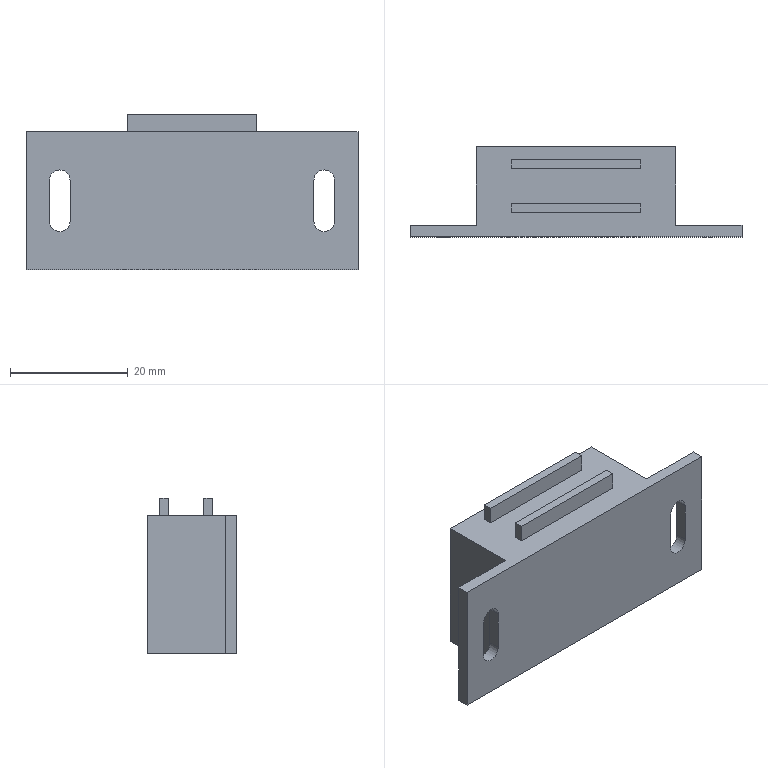Part | SolidWorks | features BaseBody 1 | 1 solid | 30 faces | box 56.5 x 15.3 x 26.5 mm | volume 13344 mm3 | plane 24 | cylinder 6 | commonest cylinder face diameters 3.5 x6
STEP:
#1=CARTESIAN_POINT('',(-20.75,0.,3.5));
#2=VERTEX_POINT('',#1);
#3=CARTESIAN_POINT('',(-22.5,0.,5.25));
#4=VERTEX_POINT('',#3);
#5=CARTESIAN_POINT('',(-22.5,0.,3.5));
#6=DIRECTION('',(0.,-1.,0.));
#7=DIRECTION('',(0.,0.,1.));
#8=AXIS2_PLACEMENT_3D('',#5,#6,#7);
#9=CIRCLE('',#8,1.75);
#10=EDGE_CURVE('',#2,#4,#9,.T.);
#11=ORIENTED_EDGE('',*,*,#10,.T.);
#12=CARTESIAN_POINT('',(-22.5,2.,5.25));
#13=VERTEX_POINT('',#12);
#14=CARTESIAN_POINT('',(-22.5,0.,5.25));
#15=DIRECTION('',(0.,1.,0.));
#16=VECTOR('',#15,1000.);
#17=LINE('',#14,#16);
#18=EDGE_CURVE('',#4,#13,#17,.T.);
#19=ORIENTED_EDGE('',*,*,#18,.T.);
#20=CARTESIAN_POINT('',(-20.75,2.,3.5));
#21=VERTEX_POINT('',#20);
#22=CARTESIAN_POINT('',(-22.5,2.,3.5));
#23=DIRECTION('',(0.,-1.,0.));
#24=DIRECTION('',(0.,0.,1.));
#25=AXIS2_PLACEMENT_3D('',#22,#23,#24);
#26=CIRCLE('',#25,1.75);
#27=EDGE_CURVE('',#21,#13,#26,.T.);
#28=ORIENTED_EDGE('',*,*,#27,.F.);
#29=CARTESIAN_POINT('',(-20.75,0.,3.5));
#30=DIRECTION('',(0.,-1.,0.));
#31=VECTOR('',#30,1000.);
#32=LINE('',#29,#31);
#33=EDGE_CURVE('',#21,#2,#32,.T.);
#34=ORIENTED_EDGE('',*,*,#33,.T.);
#35=EDGE_LOOP('',(#11,#19,#28,#34));
#36=FACE_OUTER_BOUND('',#35,.T.);
#37=CARTESIAN_POINT('',(-22.5,0.,3.5));
#38=DIRECTION('',(0.,1.,0.));
#39=DIRECTION('',(0.,0.,1.));
#40=AXIS2_PLACEMENT_3D('',#37,#38,#39);
#41=CYLINDRICAL_SURFACE('',#40,1.75);
#42=ADVANCED_FACE('',(#36),#41,.F.);
#43=CARTESIAN_POINT('',(24.25,0.,3.5));
#44=VERTEX_POINT('',#43);
#45=CARTESIAN_POINT('',(22.5,0.,5.25));
#46=VERTEX_POINT('',#45);
#47=CARTESIAN_POINT('',(22.5,0.,3.5));
#48=DIRECTION('',(0.,-1.,0.));
#49=DIRECTION('',(0.,0.,1.));
#50=AXIS2_PLACEMENT_3D('',#47,#48,#49);
#51=CIRCLE('',#50,1.75);
#52=EDGE_CURVE('',#44,#46,#51,.T.);
#53=ORIENTED_EDGE('',*,*,#52,.T.);
#54=CARTESIAN_POINT('',(22.5,2.,5.25));
#55=VERTEX_POINT('',#54);
#56=CARTESIAN_POINT('',(22.5,0.,5.25));
#57=DIRECTION('',(0.,1.,0.));
#58=VECTOR('',#57,1000.);
#59=LINE('',#56,#58);
#60=EDGE_CURVE('',#46,#55,#59,.T.);
#61=ORIENTED_EDGE('',*,*,#60,.T.);
#62=CARTESIAN_POINT('',(24.25,2.,3.5));
#63=VERTEX_POINT('',#62);
#64=CARTESIAN_POINT('',(22.5,2.,3.5));
#65=DIRECTION('',(0.,-1.,0.));
#66=DIRECTION('',(0.,0.,1.));
#67=AXIS2_PLACEMENT_3D('',#64,#65,#66);
#68=CIRCLE('',#67,1.75);
#69=EDGE_CURVE('',#63,#55,#68,.T.);
#70=ORIENTED_EDGE('',*,*,#69,.F.);
#71=CARTESIAN_POINT('',(24.25,0.,3.5));
#72=DIRECTION('',(0.,-1.,0.));
#73=VECTOR('',#72,1000.);
#74=LINE('',#71,#73);
#75=EDGE_CURVE('',#63,#44,#74,.T.);
#76=ORIENTED_EDGE('',*,*,#75,.T.);
#77=EDGE_LOOP('',(#53,#61,#70,#76));
#78=FACE_OUTER_BOUND('',#77,.T.);
#79=CARTESIAN_POINT('',(22.5,0.,3.5));
#80=DIRECTION('',(0.,1.,0.));
#81=DIRECTION('',(0.,0.,1.));
#82=AXIS2_PLACEMENT_3D('',#79,#80,#81);
#83=CYLINDRICAL_SURFACE('',#82,1.75);
#84=ADVANCED_FACE('',(#78),#83,.F.);
#85=CARTESIAN_POINT('',(-28.25,0.,11.75));
#86=VERTEX_POINT('',#85);
#87=CARTESIAN_POINT('',(28.25,0.,11.75));
#88=VERTEX_POINT('',#87);
#89=CARTESIAN_POINT('',(0.,0.,11.75));
#90=DIRECTION('',(1.,0.,0.));
#91=VECTOR('',#90,1000.);
#92=LINE('',#89,#91);
#93=EDGE_CURVE('',#86,#88,#92,.T.);
#94=ORIENTED_EDGE('',*,*,#93,.F.);
#95=CARTESIAN_POINT('',(-28.25,0.,-11.75));
#96=VERTEX_POINT('',#95);
#97=CARTESIAN_POINT('',(-28.25,0.,0.));
#98=DIRECTION('',(0.,0.,1.));
#99=VECTOR('',#98,1000.);
#100=LINE('',#97,#99);
#101=EDGE_CURVE('',#96,#86,#100,.T.);
#102=ORIENTED_EDGE('',*,*,#101,.F.);
#103=CARTESIAN_POINT('',(28.25,0.,-11.75));
#104=VERTEX_POINT('',#103);
#105=CARTESIAN_POINT('',(0.,0.,-11.75));
#106=DIRECTION('',(-1.,0.,0.));
#107=VECTOR('',#106,1000.);
#108=LINE('',#105,#107);
#109=EDGE_CURVE('',#104,#96,#108,.T.);
#110=ORIENTED_EDGE('',*,*,#109,.F.);
#111=CARTESIAN_POINT('',(28.25,0.,0.));
#112=DIRECTION('',(0.,0.,-1.));
#113=VECTOR('',#112,1000.);
#114=LINE('',#111,#113);
#115=EDGE_CURVE('',#88,#104,#114,.T.);
#116=ORIENTED_EDGE('',*,*,#115,.F.);
#117=EDGE_LOOP('',(#94,#102,#110,#116));
#118=FACE_OUTER_BOUND('',#117,.T.);
#119=CARTESIAN_POINT('',(-24.25,0.,-3.5));
#120=VERTEX_POINT('',#119);
#121=CARTESIAN_POINT('',(-20.75,0.,-3.5));
#122=VERTEX_POINT('',#121);
#123=CARTESIAN_POINT('',(-22.5,0.,-3.5));
#124=DIRECTION('',(0.,-1.,0.));
#125=DIRECTION('',(0.,0.,1.));
#126=AXIS2_PLACEMENT_3D('',#123,#124,#125);
#127=CIRCLE('',#126,1.75);
#128=EDGE_CURVE('',#120,#122,#127,.T.);
#129=ORIENTED_EDGE('',*,*,#128,.F.);
#130=CARTESIAN_POINT('',(-24.25,0.,3.5));
#131=VERTEX_POINT('',#130);
#132=CARTESIAN_POINT('',(-24.25,0.,0.));
#133=DIRECTION('',(0.,0.,-1.));
#134=VECTOR('',#133,1000.);
#135=LINE('',#132,#134);
#136=EDGE_CURVE('',#131,#120,#135,.T.);
#137=ORIENTED_EDGE('',*,*,#136,.F.);
#138=CARTESIAN_POINT('',(-22.5,0.,3.5));
#139=DIRECTION('',(0.,-1.,0.));
#140=DIRECTION('',(0.,0.,1.));
#141=AXIS2_PLACEMENT_3D('',#138,#139,#140);
#142=CIRCLE('',#141,1.75);
#143=EDGE_CURVE('',#4,#131,#142,.T.);
#144=ORIENTED_EDGE('',*,*,#143,.F.);
#145=ORIENTED_EDGE('',*,*,#10,.F.);
#146=CARTESIAN_POINT('',(-20.75,0.,0.));
#147=DIRECTION('',(0.,0.,1.));
#148=VECTOR('',#147,1000.);
#149=LINE('',#146,#148);
#150=EDGE_CURVE('',#122,#2,#149,.T.);
#151=ORIENTED_EDGE('',*,*,#150,.F.);
#152=EDGE_LOOP('',(#129,#137,#144,#145,#151));
#153=FACE_BOUND('',#152,.T.);
#154=CARTESIAN_POINT('',(20.75,0.,-3.5));
#155=VERTEX_POINT('',#154);
#156=CARTESIAN_POINT('',(24.25,0.,-3.5));
#157=VERTEX_POINT('',#156);
#158=CARTESIAN_POINT('',(22.5,0.,-3.5));
#159=DIRECTION('',(0.,-1.,0.));
#160=DIRECTION('',(0.,0.,1.));
#161=AXIS2_PLACEMENT_3D('',#158,#159,#160);
#162=CIRCLE('',#161,1.75);
#163=EDGE_CURVE('',#155,#157,#162,.T.);
#164=ORIENTED_EDGE('',*,*,#163,.F.);
#165=CARTESIAN_POINT('',(20.75,0.,3.5));
#166=VERTEX_POINT('',#165);
#167=CARTESIAN_POINT('',(20.75,0.,0.));
#168=DIRECTION('',(0.,0.,-1.));
#169=VECTOR('',#168,1000.);
#170=LINE('',#167,#169);
#171=EDGE_CURVE('',#166,#155,#170,.T.);
#172=ORIENTED_EDGE('',*,*,#171,.F.);
#173=CARTESIAN_POINT('',(22.5,0.,3.5));
#174=DIRECTION('',(0.,-1.,0.));
#175=DIRECTION('',(0.,0.,1.));
#176=AXIS2_PLACEMENT_3D('',#173,#174,#175);
#177=CIRCLE('',#176,1.75);
#178=EDGE_CURVE('',#46,#166,#177,.T.);
#179=ORIENTED_EDGE('',*,*,#178,.F.);
#180=ORIENTED_EDGE('',*,*,#52,.F.);
#181=CARTESIAN_POINT('',(24.25,0.,0.));
#182=DIRECTION('',(0.,0.,1.));
#183=VECTOR('',#182,1000.);
#184=LINE('',#181,#183);
#185=EDGE_CURVE('',#157,#44,#184,.T.);
#186=ORIENTED_EDGE('',*,*,#185,.F.);
#187=EDGE_LOOP('',(#164,#172,#179,#180,#186));
#188=FACE_BOUND('',#187,.T.);
#189=CARTESIAN_POINT('',(0.,0.,0.));
#190=DIRECTION('',(0.,1.,0.));
#191=DIRECTION('',(0.,0.,1.));
#192=AXIS2_PLACEMENT_3D('',#189,#190,#191);
#193=PLANE('',#192);
#194=ADVANCED_FACE('',(#118,#153,#188),#193,.F.);
#195=CARTESIAN_POINT('',(28.25,2.,-11.75));
#196=VERTEX_POINT('',#195);
#197=CARTESIAN_POINT('',(28.25,2.,-11.75));
#198=DIRECTION('',(0.,-1.,0.));
#199=VECTOR('',#198,1000.);
#200=LINE('',#197,#199);
#201=EDGE_CURVE('',#196,#104,#200,.T.);
#202=ORIENTED_EDGE('',*,*,#201,.F.);
#203=CARTESIAN_POINT('',(28.25,2.,11.75));
#204=VERTEX_POINT('',#203);
#205=CARTESIAN_POINT('',(28.25,2.,-11.75));
#206=DIRECTION('',(0.,0.,-1.));
#207=VECTOR('',#206,1000.);
#208=LINE('',#205,#207);
#209=EDGE_CURVE('',#204,#196,#208,.T.);
#210=ORIENTED_EDGE('',*,*,#209,.F.);
#211=CARTESIAN_POINT('',(28.25,2.,11.75));
#212=DIRECTION('',(0.,1.,0.));
#213=VECTOR('',#212,1000.);
#214=LINE('',#211,#213);
#215=EDGE_CURVE('',#88,#204,#214,.T.);
#216=ORIENTED_EDGE('',*,*,#215,.F.);
#217=ORIENTED_EDGE('',*,*,#115,.T.);
#218=EDGE_LOOP('',(#202,#210,#216,#217));
#219=FACE_OUTER_BOUND('',#218,.T.);
#220=CARTESIAN_POINT('',(28.25,2.,-11.75));
#221=DIRECTION('',(-1.,0.,0.));
#222=DIRECTION('',(0.,0.,1.));
#223=AXIS2_PLACEMENT_3D('',#220,#221,#222);
#224=PLANE('',#223);
#225=ADVANCED_FACE('',(#219),#224,.F.);
#226=CARTESIAN_POINT('',(11.,5.65,11.75));
#227=VERTEX_POINT('',#226);
#228=CARTESIAN_POINT('',(-11.,5.65,11.75));
#229=VERTEX_POINT('',#228);
#230=CARTESIAN_POINT('',(-28.25,5.65,11.75));
#231=DIRECTION('',(-1.,0.,0.));
#232=VECTOR('',#231,1000.);
#233=LINE('',#230,#232);
#234=EDGE_CURVE('',#227,#229,#233,.T.);
#235=ORIENTED_EDGE('',*,*,#234,.F.);
#236=CARTESIAN_POINT('',(11.,4.15,11.75));
#237=VERTEX_POINT('',#236);
#238=CARTESIAN_POINT('',(11.,4.15,11.75));
#239=DIRECTION('',(0.,-1.,0.));
#240=VECTOR('',#239,1000.);
#241=LINE('',#238,#240);
#242=EDGE_CURVE('',#227,#237,#241,.T.);
#243=ORIENTED_EDGE('',*,*,#242,.T.);
#244=CARTESIAN_POINT('',(-11.,4.15,11.75));
#245=VERTEX_POINT('',#244);
#246=CARTESIAN_POINT('',(-28.25,4.15,11.75));
#247=DIRECTION('',(1.,0.,0.));
#248=VECTOR('',#247,1000.);
#249=LINE('',#246,#248);
#250=EDGE_CURVE('',#245,#237,#249,.T.);
#251=ORIENTED_EDGE('',*,*,#250,.F.);
#252=CARTESIAN_POINT('',(-11.,4.15,11.75));
#253=DIRECTION('',(0.,1.,0.));
#254=VECTOR('',#253,1000.);
#255=LINE('',#252,#254);
#256=EDGE_CURVE('',#245,#229,#255,.T.);
#257=ORIENTED_EDGE('',*,*,#256,.T.);
#258=EDGE_LOOP('',(#235,#243,#251,#257));
#259=FACE_BOUND('',#258,.T.);
#260=ORIENTED_EDGE('',*,*,#215,.T.);
#261=CARTESIAN_POINT('',(17.,2.,11.75));
#262=VERTEX_POINT('',#261);
#263=CARTESIAN_POINT('',(-28.25,2.,11.75));
#264=DIRECTION('',(1.,0.,0.));
#265=VECTOR('',#264,1000.);
#266=LINE('',#263,#265);
#267=EDGE_CURVE('',#262,#204,#266,.T.);
#268=ORIENTED_EDGE('',*,*,#267,.F.);
#269=CARTESIAN_POINT('',(17.,15.3,11.75));
#270=VERTEX_POINT('',#269);
#271=CARTESIAN_POINT('',(17.,2.,11.75));
#272=DIRECTION('',(0.,-1.,0.));
#273=VECTOR('',#272,1000.);
#274=LINE('',#271,#273);
#275=EDGE_CURVE('',#270,#262,#274,.T.);
#276=ORIENTED_EDGE('',*,*,#275,.F.);
#277=CARTESIAN_POINT('',(-17.,15.3,11.75));
#278=VERTEX_POINT('',#277);
#279=CARTESIAN_POINT('',(-28.25,15.3,11.75));
#280=DIRECTION('',(1.,0.,0.));
#281=VECTOR('',#280,1000.);
#282=LINE('',#279,#281);
#283=EDGE_CURVE('',#278,#270,#282,.T.);
#284=ORIENTED_EDGE('',*,*,#283,.F.);
#285=CARTESIAN_POINT('',(-17.,2.,11.75));
#286=VERTEX_POINT('',#285);
#287=CARTESIAN_POINT('',(-17.,2.,11.75));
#288=DIRECTION('',(0.,1.,0.));
#289=VECTOR('',#288,1000.);
#290=LINE('',#287,#289);
#291=EDGE_CURVE('',#286,#278,#290,.T.);
#292=ORIENTED_EDGE('',*,*,#291,.F.);
#293=CARTESIAN_POINT('',(-28.25,2.,11.75));
#294=VERTEX_POINT('',#293);
#295=CARTESIAN_POINT('',(-28.25,2.,11.75));
#296=DIRECTION('',(1.,0.,0.));
#297=VECTOR('',#296,1000.);
#298=LINE('',#295,#297);
#299=EDGE_CURVE('',#294,#286,#298,.T.);
#300=ORIENTED_EDGE('',*,*,#299,.F.);
#301=CARTESIAN_POINT('',(-28.25,2.,11.75));
#302=DIRECTION('',(0.,1.,0.));
#303=VECTOR('',#302,1000.);
#304=LINE('',#301,#303);
#305=EDGE_CURVE('',#86,#294,#304,.T.);
#306=ORIENTED_EDGE('',*,*,#305,.F.);
#307=ORIENTED_EDGE('',*,*,#93,.T.);
#308=EDGE_LOOP('',(#260,#268,#276,#284,#292,#300,#306,#307));
#309=FACE_OUTER_BOUND('',#308,.T.);
#310=CARTESIAN_POINT('',(-11.,11.65,11.75));
#311=VERTEX_POINT('',#310);
#312=CARTESIAN_POINT('',(11.,11.65,11.75));
#313=VERTEX_POINT('',#312);
#314=CARTESIAN_POINT('',(-28.25,11.65,11.75));
#315=DIRECTION('',(1.,0.,0.));
#316=VECTOR('',#315,1000.);
#317=LINE('',#314,#316);
#318=EDGE_CURVE('',#311,#313,#317,.T.);
#319=ORIENTED_EDGE('',*,*,#318,.F.);
#320=CARTESIAN_POINT('',(-11.,13.15,11.75));
#321=VERTEX_POINT('',#320);
#322=CARTESIAN_POINT('',(-11.,13.15,11.75));
#323=DIRECTION('',(0.,1.,0.));
#324=VECTOR('',#323,1000.);
#325=LINE('',#322,#324);
#326=EDGE_CURVE('',#311,#321,#325,.T.);
#327=ORIENTED_EDGE('',*,*,#326,.T.);
#328=CARTESIAN_POINT('',(11.,13.15,11.75));
#329=VERTEX_POINT('',#328);
#330=CARTESIAN_POINT('',(-28.25,13.15,11.75));
#331=DIRECTION('',(-1.,0.,0.));
#332=VECTOR('',#331,1000.);
#333=LINE('',#330,#332);
#334=EDGE_CURVE('',#329,#321,#333,.T.);
#335=ORIENTED_EDGE('',*,*,#334,.F.);
#336=CARTESIAN_POINT('',(11.,13.15,11.75));
#337=DIRECTION('',(0.,-1.,0.));
#338=VECTOR('',#337,1000.);
#339=LINE('',#336,#338);
#340=EDGE_CURVE('',#329,#313,#339,.T.);
#341=ORIENTED_EDGE('',*,*,#340,.T.);
#342=EDGE_LOOP('',(#319,#327,#335,#341));
#343=FACE_BOUND('',#342,.T.);
#344=CARTESIAN_POINT('',(-28.25,2.,11.75));
#345=DIRECTION('',(0.,0.,-1.));
#346=DIRECTION('',(-1.,0.,0.));
#347=AXIS2_PLACEMENT_3D('',#344,#345,#346);
#348=PLANE('',#347);
#349=ADVANCED_FACE('',(#259,#309,#343),#348,.F.);
#350=ORIENTED_EDGE('',*,*,#305,.T.);
#351=CARTESIAN_POINT('',(-28.25,2.,-11.75));
#352=VERTEX_POINT('',#351);
#353=CARTESIAN_POINT('',(-28.25,2.,-11.75));
#354=DIRECTION('',(0.,0.,1.));
#355=VECTOR('',#354,1000.);
#356=LINE('',#353,#355);
#357=EDGE_CURVE('',#352,#294,#356,.T.);
#358=ORIENTED_EDGE('',*,*,#357,.F.);
#359=CARTESIAN_POINT('',(-28.25,2.,-11.75));
#360=DIRECTION('',(0.,1.,0.));
#361=VECTOR('',#360,1000.);
#362=LINE('',#359,#361);
#363=EDGE_CURVE('',#96,#352,#362,.T.);
#364=ORIENTED_EDGE('',*,*,#363,.F.);
#365=ORIENTED_EDGE('',*,*,#101,.T.);
#366=EDGE_LOOP('',(#350,#358,#364,#365));
#367=FACE_OUTER_BOUND('',#366,.T.);
#368=CARTESIAN_POINT('',(-28.25,2.,-11.75));
#369=DIRECTION('',(1.,0.,0.));
#370=DIRECTION('',(0.,0.,-1.));
#371=AXIS2_PLACEMENT_3D('',#368,#369,#370);
#372=PLANE('',#371);
#373=ADVANCED_FACE('',(#367),#372,.F.);
#374=ORIENTED_EDGE('',*,*,#363,.T.);
#375=CARTESIAN_POINT('',(-17.,2.,-11.75));
#376=VERTEX_POINT('',#375);
#377=CARTESIAN_POINT('',(-28.25,2.,-11.75));
#378=DIRECTION('',(-1.,0.,0.));
#379=VECTOR('',#378,1000.);
#380=LINE('',#377,#379);
#381=EDGE_CURVE('',#376,#352,#380,.T.);
#382=ORIENTED_EDGE('',*,*,#381,.F.);
#383=CARTESIAN_POINT('',(-17.,15.3,-11.75));
#384=VERTEX_POINT('',#383);
#385=CARTESIAN_POINT('',(-17.,2.,-11.75));
#386=DIRECTION('',(0.,-1.,0.));
#387=VECTOR('',#386,1000.);
#388=LINE('',#385,#387);
#389=EDGE_CURVE('',#384,#376,#388,.T.);
#390=ORIENTED_EDGE('',*,*,#389,.F.);
#391=CARTESIAN_POINT('',(17.,15.3,-11.75));
#392=VERTEX_POINT('',#391);
#393=CARTESIAN_POINT('',(-28.25,15.3,-11.75));
#394=DIRECTION('',(-1.,0.,0.));
#395=VECTOR('',#394,1000.);
#396=LINE('',#393,#395);
#397=EDGE_CURVE('',#392,#384,#396,.T.);
#398=ORIENTED_EDGE('',*,*,#397,.F.);
#399=CARTESIAN_POINT('',(17.,2.,-11.75));
#400=VERTEX_POINT('',#399);
#401=CARTESIAN_POINT('',(17.,2.,-11.75));
#402=DIRECTION('',(0.,1.,0.));
#403=VECTOR('',#402,1000.);
#404=LINE('',#401,#403);
#405=EDGE_CURVE('',#400,#392,#404,.T.);
#406=ORIENTED_EDGE('',*,*,#405,.F.);
#407=CARTESIAN_POINT('',(-28.25,2.,-11.75));
#408=DIRECTION('',(-1.,0.,0.));
#409=VECTOR('',#408,1000.);
#410=LINE('',#407,#409);
#411=EDGE_CURVE('',#196,#400,#410,.T.);
#412=ORIENTED_EDGE('',*,*,#411,.F.);
#413=ORIENTED_EDGE('',*,*,#201,.T.);
#414=ORIENTED_EDGE('',*,*,#109,.T.);
#415=EDGE_LOOP('',(#374,#382,#390,#398,#406,#412,#413,#414));
#416=FACE_OUTER_BOUND('',#415,.T.);
#417=CARTESIAN_POINT('',(-28.25,2.,-11.75));
#418=DIRECTION('',(0.,0.,1.));
#419=DIRECTION('',(1.,0.,0.));
#420=AXIS2_PLACEMENT_3D('',#417,#418,#419);
#421=PLANE('',#420);
#422=ADVANCED_FACE('',(#416),#421,.F.);
#423=CARTESIAN_POINT('',(-20.75,2.,-3.5));
#424=VERTEX_POINT('',#423);
#425=CARTESIAN_POINT('',(-20.75,0.,-3.5));
#426=DIRECTION('',(0.,1.,0.));
#427=VECTOR('',#426,1000.);
#428=LINE('',#425,#427);
#429=EDGE_CURVE('',#122,#424,#428,.T.);
#430=ORIENTED_EDGE('',*,*,#429,.F.);
#431=ORIENTED_EDGE('',*,*,#150,.T.);
#432=ORIENTED_EDGE('',*,*,#33,.F.);
#433=CARTESIAN_POINT('',(-20.75,2.,-3.5));
#434=DIRECTION('',(0.,0.,1.));
#435=VECTOR('',#434,1000.);
#436=LINE('',#433,#435);
#437=EDGE_CURVE('',#424,#21,#436,.T.);
#438=ORIENTED_EDGE('',*,*,#437,.F.);
#439=EDGE_LOOP('',(#430,#431,#432,#438));
#440=FACE_OUTER_BOUND('',#439,.T.);
#441=CARTESIAN_POINT('',(-20.75,0.,-3.5));
#442=DIRECTION('',(1.,0.,0.));
#443=DIRECTION('',(0.,0.,-1.));
#444=AXIS2_PLACEMENT_3D('',#441,#442,#443);
#445=PLANE('',#444);
#446=ADVANCED_FACE('',(#440),#445,.F.);
#447=CARTESIAN_POINT('',(-24.25,2.,-3.5));
#448=VERTEX_POINT('',#447);
#449=CARTESIAN_POINT('',(-24.25,0.,-3.5));
#450=DIRECTION('',(0.,1.,0.));
#451=VECTOR('',#450,1000.);
#452=LINE('',#449,#451);
#453=EDGE_CURVE('',#120,#448,#452,.T.);
#454=ORIENTED_EDGE('',*,*,#453,.F.);
#455=ORIENTED_EDGE('',*,*,#128,.T.);
#456=ORIENTED_EDGE('',*,*,#429,.T.);
#457=CARTESIAN_POINT('',(-22.5,2.,-3.5));
#458=DIRECTION('',(0.,-1.,0.));
#459=DIRECTION('',(0.,0.,1.));
#460=AXIS2_PLACEMENT_3D('',#457,#458,#459);
#461=CIRCLE('',#460,1.75);
#462=EDGE_CURVE('',#448,#424,#461,.T.);
#463=ORIENTED_EDGE('',*,*,#462,.F.);
#464=EDGE_LOOP('',(#454,#455,#456,#463));
#465=FACE_OUTER_BOUND('',#464,.T.);
#466=CARTESIAN_POINT('',(-22.5,0.,-3.5));
#467=DIRECTION('',(0.,1.,0.));
#468=DIRECTION('',(0.,0.,1.));
#469=AXIS2_PLACEMENT_3D('',#466,#467,#468);
#470=CYLINDRICAL_SURFACE('',#469,1.75);
#471=ADVANCED_FACE('',(#465),#470,.F.);
#472=CARTESIAN_POINT('',(-24.25,2.,3.5));
#473=VERTEX_POINT('',#472);
#474=CARTESIAN_POINT('',(-24.25,0.,3.5));
#475=DIRECTION('',(0.,1.,0.));
#476=VECTOR('',#475,1000.);
#477=LINE('',#474,#476);
#478=EDGE_CURVE('',#131,#473,#477,.T.);
#479=ORIENTED_EDGE('',*,*,#478,.F.);
#480=ORIENTED_EDGE('',*,*,#136,.T.);
#481=ORIENTED_EDGE('',*,*,#453,.T.);
#482=CARTESIAN_POINT('',(-24.25,2.,-3.5));
#483=DIRECTION('',(0.,0.,-1.));
#484=VECTOR('',#483,1000.);
#485=LINE('',#482,#484);
#486=EDGE_CURVE('',#473,#448,#485,.T.);
#487=ORIENTED_EDGE('',*,*,#486,.F.);
#488=EDGE_LOOP('',(#479,#480,#481,#487));
#489=FACE_OUTER_BOUND('',#488,.T.);
#490=CARTESIAN_POINT('',(-24.25,0.,-3.5));
#491=DIRECTION('',(-1.,0.,0.));
#492=DIRECTION('',(0.,0.,1.));
#493=AXIS2_PLACEMENT_3D('',#490,#491,#492);
#494=PLANE('',#493);
#495=ADVANCED_FACE('',(#489),#494,.F.);
#496=ORIENTED_EDGE('',*,*,#18,.F.);
#497=ORIENTED_EDGE('',*,*,#143,.T.);
#498=ORIENTED_EDGE('',*,*,#478,.T.);
#499=CARTESIAN_POINT('',(-22.5,2.,3.5));
#500=DIRECTION('',(0.,-1.,0.));
#501=DIRECTION('',(0.,0.,1.));
#502=AXIS2_PLACEMENT_3D('',#499,#500,#501);
#503=CIRCLE('',#502,1.75);
#504=EDGE_CURVE('',#13,#473,#503,.T.);
#505=ORIENTED_EDGE('',*,*,#504,.F.);
#506=EDGE_LOOP('',(#496,#497,#498,#505));
#507=FACE_OUTER_BOUND('',#506,.T.);
#508=CARTESIAN_POINT('',(-22.5,0.,3.5));
#509=DIRECTION('',(0.,1.,0.));
#510=DIRECTION('',(0.,0.,1.));
#511=AXIS2_PLACEMENT_3D('',#508,#509,#510);
#512=CYLINDRICAL_SURFACE('',#511,1.75);
#513=ADVANCED_FACE('',(#507),#512,.F.);
#514=CARTESIAN_POINT('',(24.25,2.,-3.5));
#515=VERTEX_POINT('',#514);
#516=CARTESIAN_POINT('',(24.25,0.,-3.5));
#517=DIRECTION('',(0.,1.,0.));
#518=VECTOR('',#517,1000.);
#519=LINE('',#516,#518);
#520=EDGE_CURVE('',#157,#515,#519,.T.);
#521=ORIENTED_EDGE('',*,*,#520,.F.);
#522=ORIENTED_EDGE('',*,*,#185,.T.);
#523=ORIENTED_EDGE('',*,*,#75,.F.);
#524=CARTESIAN_POINT('',(24.25,2.,-3.5));
#525=DIRECTION('',(0.,0.,1.));
#526=VECTOR('',#525,1000.);
#527=LINE('',#524,#526);
#528=EDGE_CURVE('',#515,#63,#527,.T.);
#529=ORIENTED_EDGE('',*,*,#528,.F.);
#530=EDGE_LOOP('',(#521,#522,#523,#529));
#531=FACE_OUTER_BOUND('',#530,.T.);
#532=CARTESIAN_POINT('',(24.25,0.,-3.5));
#533=DIRECTION('',(1.,0.,0.));
#534=DIRECTION('',(0.,0.,-1.));
#535=AXIS2_PLACEMENT_3D('',#532,#533,#534);
#536=PLANE('',#535);
#537=ADVANCED_FACE('',(#531),#536,.F.);
#538=CARTESIAN_POINT('',(20.75,2.,-3.5));
#539=VERTEX_POINT('',#538);
#540=CARTESIAN_POINT('',(20.75,0.,-3.5));
#541=DIRECTION('',(0.,1.,0.));
#542=VECTOR('',#541,1000.);
#543=LINE('',#540,#542);
#544=EDGE_CURVE('',#155,#539,#543,.T.);
#545=ORIENTED_EDGE('',*,*,#544,.F.);
#546=ORIENTED_EDGE('',*,*,#163,.T.);
#547=ORIENTED_EDGE('',*,*,#520,.T.);
#548=CARTESIAN_POINT('',(22.5,2.,-3.5));
#549=DIRECTION('',(0.,-1.,0.));
#550=DIRECTION('',(0.,0.,1.));
#551=AXIS2_PLACEMENT_3D('',#548,#549,#550);
#552=CIRCLE('',#551,1.75);
#553=EDGE_CURVE('',#539,#515,#552,.T.);
#554=ORIENTED_EDGE('',*,*,#553,.F.);
#555=EDGE_LOOP('',(#545,#546,#547,#554));
#556=FACE_OUTER_BOUND('',#555,.T.);
#557=CARTESIAN_POINT('',(22.5,0.,-3.5));
#558=DIRECTION('',(0.,1.,0.));
#559=DIRECTION('',(0.,0.,1.));
#560=AXIS2_PLACEMENT_3D('',#557,#558,#559);
#561=CYLINDRICAL_SURFACE('',#560,1.75);
#562=ADVANCED_FACE('',(#556),#561,.F.);
#563=CARTESIAN_POINT('',(20.75,2.,3.5));
#564=VERTEX_POINT('',#563);
#565=CARTESIAN_POINT('',(20.75,0.,3.5));
#566=DIRECTION('',(0.,1.,0.));
#567=VECTOR('',#566,1000.);
#568=LINE('',#565,#567);
#569=EDGE_CURVE('',#166,#564,#568,.T.);
#570=ORIENTED_EDGE('',*,*,#569,.F.);
#571=ORIENTED_EDGE('',*,*,#171,.T.);
#572=ORIENTED_EDGE('',*,*,#544,.T.);
#573=CARTESIAN_POINT('',(20.75,2.,-3.5));
#574=DIRECTION('',(0.,0.,-1.));
#575=VECTOR('',#574,1000.);
#576=LINE('',#573,#575);
#577=EDGE_CURVE('',#564,#539,#576,.T.);
#578=ORIENTED_EDGE('',*,*,#577,.F.);
#579=EDGE_LOOP('',(#570,#571,#572,#578));
#580=FACE_OUTER_BOUND('',#579,.T.);
#581=CARTESIAN_POINT('',(20.75,0.,-3.5));
#582=DIRECTION('',(-1.,0.,0.));
#583=DIRECTION('',(0.,0.,1.));
#584=AXIS2_PLACEMENT_3D('',#581,#582,#583);
#585=PLANE('',#584);
#586=ADVANCED_FACE('',(#580),#585,.F.);
#587=ORIENTED_EDGE('',*,*,#60,.F.);
#588=ORIENTED_EDGE('',*,*,#178,.T.);
#589=ORIENTED_EDGE('',*,*,#569,.T.);
#590=CARTESIAN_POINT('',(22.5,2.,3.5));
#591=DIRECTION('',(0.,-1.,0.));
#592=DIRECTION('',(0.,0.,1.));
#593=AXIS2_PLACEMENT_3D('',#590,#591,#592);
#594=CIRCLE('',#593,1.75);
#595=EDGE_CURVE('',#55,#564,#594,.T.);
#596=ORIENTED_EDGE('',*,*,#595,.F.);
#597=EDGE_LOOP('',(#587,#588,#589,#596));
#598=FACE_OUTER_BOUND('',#597,.T.);
#599=CARTESIAN_POINT('',(22.5,0.,3.5));
#600=DIRECTION('',(0.,1.,0.));
#601=DIRECTION('',(0.,0.,1.));
#602=AXIS2_PLACEMENT_3D('',#599,#600,#601);
#603=CYLINDRICAL_SURFACE('',#602,1.75);
#604=ADVANCED_FACE('',(#598),#603,.F.);
#605=ORIENTED_EDGE('',*,*,#209,.T.);
#606=ORIENTED_EDGE('',*,*,#411,.T.);
#607=CARTESIAN_POINT('',(17.,2.,0.));
#608=DIRECTION('',(0.,0.,1.));
#609=VECTOR('',#608,1000.);
#610=LINE('',#607,#609);
#611=EDGE_CURVE('',#400,#262,#610,.T.);
#612=ORIENTED_EDGE('',*,*,#611,.T.);
#613=ORIENTED_EDGE('',*,*,#267,.T.);
#614=EDGE_LOOP('',(#605,#606,#612,#613));
#615=FACE_OUTER_BOUND('',#614,.T.);
#616=ORIENTED_EDGE('',*,*,#69,.T.);
#617=ORIENTED_EDGE('',*,*,#595,.T.);
#618=ORIENTED_EDGE('',*,*,#577,.T.);
#619=ORIENTED_EDGE('',*,*,#553,.T.);
#620=ORIENTED_EDGE('',*,*,#528,.T.);
#621=EDGE_LOOP('',(#616,#617,#618,#619,#620));
#622=FACE_BOUND('',#621,.T.);
#623=CARTESIAN_POINT('',(0.,2.,0.));
#624=DIRECTION('',(0.,1.,0.));
#625=DIRECTION('',(0.,0.,1.));
#626=AXIS2_PLACEMENT_3D('',#623,#624,#625);
#627=PLANE('',#626);
#628=ADVANCED_FACE('',(#615,#622),#627,.T.);
#629=CARTESIAN_POINT('',(-11.,5.65,14.75));
#630=VERTEX_POINT('',#629);
#631=CARTESIAN_POINT('',(-11.,5.65,14.75));
#632=DIRECTION('',(0.,0.,-1.));
#633=VECTOR('',#632,1000.);
#634=LINE('',#631,#633);
#635=EDGE_CURVE('',#630,#229,#634,.T.);
#636=ORIENTED_EDGE('',*,*,#635,.F.);
#637=CARTESIAN_POINT('',(11.,5.65,14.75));
#638=VERTEX_POINT('',#637);
#639=CARTESIAN_POINT('',(-11.,5.65,14.75));
#640=DIRECTION('',(-1.,0.,0.));
#641=VECTOR('',#640,1000.);
#642=LINE('',#639,#641);
#643=EDGE_CURVE('',#638,#630,#642,.T.);
#644=ORIENTED_EDGE('',*,*,#643,.F.);
#645=CARTESIAN_POINT('',(11.,5.65,14.75));
#646=DIRECTION('',(0.,0.,1.));
#647=VECTOR('',#646,1000.);
#648=LINE('',#645,#647);
#649=EDGE_CURVE('',#227,#638,#648,.T.);
#650=ORIENTED_EDGE('',*,*,#649,.F.);
#651=ORIENTED_EDGE('',*,*,#234,.T.);
#652=EDGE_LOOP('',(#636,#644,#650,#651));
#653=FACE_OUTER_BOUND('',#652,.T.);
#654=CARTESIAN_POINT('',(-11.,5.65,14.75));
#655=DIRECTION('',(0.,-1.,0.));
#656=DIRECTION('',(0.,0.,-1.));
#657=AXIS2_PLACEMENT_3D('',#654,#655,#656);
#658=PLANE('',#657);
#659=ADVANCED_FACE('',(#653),#658,.F.);
#660=CARTESIAN_POINT('',(11.,4.15,14.75));
#661=VERTEX_POINT('',#660);
#662=CARTESIAN_POINT('',(11.,4.15,14.75));
#663=DIRECTION('',(0.,0.,-1.));
#664=VECTOR('',#663,1000.);
#665=LINE('',#662,#664);
#666=EDGE_CURVE('',#661,#237,#665,.T.);
#667=ORIENTED_EDGE('',*,*,#666,.F.);
#668=CARTESIAN_POINT('',(-11.,4.15,14.75));
#669=VERTEX_POINT('',#668);
#670=CARTESIAN_POINT('',(-11.,4.15,14.75));
#671=DIRECTION('',(1.,0.,0.));
#672=VECTOR('',#671,1000.);
#673=LINE('',#670,#672);
#674=EDGE_CURVE('',#669,#661,#673,.T.);
#675=ORIENTED_EDGE('',*,*,#674,.F.);
#676=CARTESIAN_POINT('',(-11.,4.15,14.75));
#677=DIRECTION('',(0.,0.,1.));
#678=VECTOR('',#677,1000.);
#679=LINE('',#676,#678);
#680=EDGE_CURVE('',#245,#669,#679,.T.);
#681=ORIENTED_EDGE('',*,*,#680,.F.);
#682=ORIENTED_EDGE('',*,*,#250,.T.);
#683=EDGE_LOOP('',(#667,#675,#681,#682));
#684=FACE_OUTER_BOUND('',#683,.T.);
#685=CARTESIAN_POINT('',(-11.,4.15,14.75));
#686=DIRECTION('',(0.,1.,0.));
#687=DIRECTION('',(-1.,0.,0.));
#688=AXIS2_PLACEMENT_3D('',#685,#686,#687);
#689=PLANE('',#688);
#690=ADVANCED_FACE('',(#684),#689,.F.);
#691=ORIENTED_EDGE('',*,*,#405,.T.);
#692=CARTESIAN_POINT('',(17.,15.3,-11.75));
#693=DIRECTION('',(0.,0.,-1.));
#694=VECTOR('',#693,1000.);
#695=LINE('',#692,#694);
#696=EDGE_CURVE('',#270,#392,#695,.T.);
#697=ORIENTED_EDGE('',*,*,#696,.F.);
#698=ORIENTED_EDGE('',*,*,#275,.T.);
#699=ORIENTED_EDGE('',*,*,#611,.F.);
#700=EDGE_LOOP('',(#691,#697,#698,#699));
#701=FACE_OUTER_BOUND('',#700,.T.);
#702=CARTESIAN_POINT('',(17.,15.3,-11.75));
#703=DIRECTION('',(-1.,0.,0.));
#704=DIRECTION('',(0.,0.,1.));
#705=AXIS2_PLACEMENT_3D('',#702,#703,#704);
#706=PLANE('',#705);
#707=ADVANCED_FACE('',(#701),#706,.F.);
#708=CARTESIAN_POINT('',(-17.,15.3,0.));
#709=DIRECTION('',(0.,0.,1.));
#710=VECTOR('',#709,1000.);
#711=LINE('',#708,#710);
#712=EDGE_CURVE('',#384,#278,#711,.T.);
#713=ORIENTED_EDGE('',*,*,#712,.T.);
#714=ORIENTED_EDGE('',*,*,#283,.T.);
#715=ORIENTED_EDGE('',*,*,#696,.T.);
#716=ORIENTED_EDGE('',*,*,#397,.T.);
#717=EDGE_LOOP('',(#713,#714,#715,#716));
#718=FACE_OUTER_BOUND('',#717,.T.);
#719=CARTESIAN_POINT('',(0.,15.3,0.));
#720=DIRECTION('',(0.,1.,0.));
#721=DIRECTION('',(0.,0.,1.));
#722=AXIS2_PLACEMENT_3D('',#719,#720,#721);
#723=PLANE('',#722);
#724=ADVANCED_FACE('',(#718),#723,.T.);
#725=ORIENTED_EDGE('',*,*,#291,.T.);
#726=ORIENTED_EDGE('',*,*,#712,.F.);
#727=ORIENTED_EDGE('',*,*,#389,.T.);
#728=CARTESIAN_POINT('',(-17.,2.,-11.75));
#729=DIRECTION('',(0.,0.,-1.));
#730=VECTOR('',#729,1000.);
#731=LINE('',#728,#730);
#732=EDGE_CURVE('',#286,#376,#731,.T.);
#733=ORIENTED_EDGE('',*,*,#732,.F.);
#734=EDGE_LOOP('',(#725,#726,#727,#733));
#735=FACE_OUTER_BOUND('',#734,.T.);
#736=CARTESIAN_POINT('',(-17.,15.3,-11.75));
#737=DIRECTION('',(1.,0.,0.));
#738=DIRECTION('',(0.,0.,-1.));
#739=AXIS2_PLACEMENT_3D('',#736,#737,#738);
#740=PLANE('',#739);
#741=ADVANCED_FACE('',(#735),#740,.F.);
#742=ORIENTED_EDGE('',*,*,#357,.T.);
#743=ORIENTED_EDGE('',*,*,#299,.T.);
#744=ORIENTED_EDGE('',*,*,#732,.T.);
#745=ORIENTED_EDGE('',*,*,#381,.T.);
#746=EDGE_LOOP('',(#742,#743,#744,#745));
#747=FACE_OUTER_BOUND('',#746,.T.);
#748=ORIENTED_EDGE('',*,*,#27,.T.);
#749=ORIENTED_EDGE('',*,*,#504,.T.);
#750=ORIENTED_EDGE('',*,*,#486,.T.);
#751=ORIENTED_EDGE('',*,*,#462,.T.);
#752=ORIENTED_EDGE('',*,*,#437,.T.);
#753=EDGE_LOOP('',(#748,#749,#750,#751,#752));
#754=FACE_BOUND('',#753,.T.);
#755=CARTESIAN_POINT('',(0.,2.,0.));
#756=DIRECTION('',(0.,1.,0.));
#757=DIRECTION('',(0.,0.,1.));
#758=AXIS2_PLACEMENT_3D('',#755,#756,#757);
#759=PLANE('',#758);
#760=ADVANCED_FACE('',(#747,#754),#759,.T.);
#761=CARTESIAN_POINT('',(11.,11.65,14.75));
#762=VERTEX_POINT('',#761);
#763=CARTESIAN_POINT('',(11.,11.65,14.75));
#764=DIRECTION('',(0.,0.,-1.));
#765=VECTOR('',#764,1000.);
#766=LINE('',#763,#765);
#767=EDGE_CURVE('',#762,#313,#766,.T.);
#768=ORIENTED_EDGE('',*,*,#767,.F.);
#769=CARTESIAN_POINT('',(-11.,11.65,14.75));
#770=VERTEX_POINT('',#769);
#771=CARTESIAN_POINT('',(-11.,11.65,14.75));
#772=DIRECTION('',(1.,0.,0.));
#773=VECTOR('',#772,1000.);
#774=LINE('',#771,#773);
#775=EDGE_CURVE('',#770,#762,#774,.T.);
#776=ORIENTED_EDGE('',*,*,#775,.F.);
#777=CARTESIAN_POINT('',(-11.,11.65,14.75));
#778=DIRECTION('',(0.,0.,1.));
#779=VECTOR('',#778,1000.);
#780=LINE('',#777,#779);
#781=EDGE_CURVE('',#311,#770,#780,.T.);
#782=ORIENTED_EDGE('',*,*,#781,.F.);
#783=ORIENTED_EDGE('',*,*,#318,.T.);
#784=EDGE_LOOP('',(#768,#776,#782,#783));
#785=FACE_OUTER_BOUND('',#784,.T.);
#786=CARTESIAN_POINT('',(-11.,11.65,14.75));
#787=DIRECTION('',(0.,1.,0.));
#788=DIRECTION('',(0.,0.,1.));
#789=AXIS2_PLACEMENT_3D('',#786,#787,#788);
#790=PLANE('',#789);
#791=ADVANCED_FACE('',(#785),#790,.F.);
#792=CARTESIAN_POINT('',(-11.,13.15,14.75));
#793=VERTEX_POINT('',#792);
#794=CARTESIAN_POINT('',(-11.,13.15,14.75));
#795=DIRECTION('',(0.,0.,-1.));
#796=VECTOR('',#795,1000.);
#797=LINE('',#794,#796);
#798=EDGE_CURVE('',#793,#321,#797,.T.);
#799=ORIENTED_EDGE('',*,*,#798,.F.);
#800=CARTESIAN_POINT('',(11.,13.15,14.75));
#801=VERTEX_POINT('',#800);
#802=CARTESIAN_POINT('',(-11.,13.15,14.75));
#803=DIRECTION('',(-1.,0.,0.));
#804=VECTOR('',#803,1000.);
#805=LINE('',#802,#804);
#806=EDGE_CURVE('',#801,#793,#805,.T.);
#807=ORIENTED_EDGE('',*,*,#806,.F.);
#808=CARTESIAN_POINT('',(11.,13.15,14.75));
#809=DIRECTION('',(0.,0.,1.));
#810=VECTOR('',#809,1000.);
#811=LINE('',#808,#810);
#812=EDGE_CURVE('',#329,#801,#811,.T.);
#813=ORIENTED_EDGE('',*,*,#812,.F.);
#814=ORIENTED_EDGE('',*,*,#334,.T.);
#815=EDGE_LOOP('',(#799,#807,#813,#814));
#816=FACE_OUTER_BOUND('',#815,.T.);
#817=CARTESIAN_POINT('',(-11.,13.15,14.75));
#818=DIRECTION('',(0.,-1.,0.));
#819=DIRECTION('',(1.,0.,0.));
#820=AXIS2_PLACEMENT_3D('',#817,#818,#819);
#821=PLANE('',#820);
#822=ADVANCED_FACE('',(#816),#821,.F.);
#823=ORIENTED_EDGE('',*,*,#680,.T.);
#824=CARTESIAN_POINT('',(-11.,4.15,14.75));
#825=DIRECTION('',(0.,-1.,0.));
#826=VECTOR('',#825,1000.);
#827=LINE('',#824,#826);
#828=EDGE_CURVE('',#630,#669,#827,.T.);
#829=ORIENTED_EDGE('',*,*,#828,.F.);
#830=ORIENTED_EDGE('',*,*,#635,.T.);
#831=ORIENTED_EDGE('',*,*,#256,.F.);
#832=EDGE_LOOP('',(#823,#829,#830,#831));
#833=FACE_OUTER_BOUND('',#832,.T.);
#834=CARTESIAN_POINT('',(-11.,4.15,14.75));
#835=DIRECTION('',(1.,0.,0.));
#836=DIRECTION('',(0.,0.,-1.));
#837=AXIS2_PLACEMENT_3D('',#834,#835,#836);
#838=PLANE('',#837);
#839=ADVANCED_FACE('',(#833),#838,.F.);
#840=ORIENTED_EDGE('',*,*,#674,.T.);
#841=CARTESIAN_POINT('',(11.,0.,14.75));
#842=DIRECTION('',(0.,-1.,0.));
#843=VECTOR('',#842,1000.);
#844=LINE('',#841,#843);
#845=EDGE_CURVE('',#638,#661,#844,.T.);
#846=ORIENTED_EDGE('',*,*,#845,.F.);
#847=ORIENTED_EDGE('',*,*,#643,.T.);
#848=ORIENTED_EDGE('',*,*,#828,.T.);
#849=EDGE_LOOP('',(#840,#846,#847,#848));
#850=FACE_OUTER_BOUND('',#849,.T.);
#851=CARTESIAN_POINT('',(0.,0.,14.75));
#852=DIRECTION('',(0.,0.,-1.));
#853=DIRECTION('',(-1.,0.,0.));
#854=AXIS2_PLACEMENT_3D('',#851,#852,#853);
#855=PLANE('',#854);
#856=ADVANCED_FACE('',(#850),#855,.F.);
#857=ORIENTED_EDGE('',*,*,#649,.T.);
#858=ORIENTED_EDGE('',*,*,#845,.T.);
#859=ORIENTED_EDGE('',*,*,#666,.T.);
#860=ORIENTED_EDGE('',*,*,#242,.F.);
#861=EDGE_LOOP('',(#857,#858,#859,#860));
#862=FACE_OUTER_BOUND('',#861,.T.);
#863=CARTESIAN_POINT('',(11.,4.15,14.75));
#864=DIRECTION('',(-1.,0.,0.));
#865=DIRECTION('',(0.,0.,1.));
#866=AXIS2_PLACEMENT_3D('',#863,#864,#865);
#867=PLANE('',#866);
#868=ADVANCED_FACE('',(#862),#867,.F.);
#869=ORIENTED_EDGE('',*,*,#812,.T.);
#870=CARTESIAN_POINT('',(11.,13.15,14.75));
#871=DIRECTION('',(0.,1.,0.));
#872=VECTOR('',#871,1000.);
#873=LINE('',#870,#872);
#874=EDGE_CURVE('',#762,#801,#873,.T.);
#875=ORIENTED_EDGE('',*,*,#874,.F.);
#876=ORIENTED_EDGE('',*,*,#767,.T.);
#877=ORIENTED_EDGE('',*,*,#340,.F.);
#878=EDGE_LOOP('',(#869,#875,#876,#877));
#879=FACE_OUTER_BOUND('',#878,.T.);
#880=CARTESIAN_POINT('',(11.,13.15,14.75));
#881=DIRECTION('',(-1.,0.,0.));
#882=DIRECTION('',(0.,0.,1.));
#883=AXIS2_PLACEMENT_3D('',#880,#881,#882);
#884=PLANE('',#883);
#885=ADVANCED_FACE('',(#879),#884,.F.);
#886=CARTESIAN_POINT('',(-11.,0.,14.75));
#887=DIRECTION('',(0.,-1.,0.));
#888=VECTOR('',#887,1000.);
#889=LINE('',#886,#888);
#890=EDGE_CURVE('',#793,#770,#889,.T.);
#891=ORIENTED_EDGE('',*,*,#890,.T.);
#892=ORIENTED_EDGE('',*,*,#775,.T.);
#893=ORIENTED_EDGE('',*,*,#874,.T.);
#894=ORIENTED_EDGE('',*,*,#806,.T.);
#895=EDGE_LOOP('',(#891,#892,#893,#894));
#896=FACE_OUTER_BOUND('',#895,.T.);
#897=CARTESIAN_POINT('',(0.,0.,14.75));
#898=DIRECTION('',(0.,0.,1.));
#899=DIRECTION('',(1.,0.,0.));
#900=AXIS2_PLACEMENT_3D('',#897,#898,#899);
#901=PLANE('',#900);
#902=ADVANCED_FACE('',(#896),#901,.T.);
#903=ORIENTED_EDGE('',*,*,#781,.T.);
#904=ORIENTED_EDGE('',*,*,#890,.F.);
#905=ORIENTED_EDGE('',*,*,#798,.T.);
#906=ORIENTED_EDGE('',*,*,#326,.F.);
#907=EDGE_LOOP('',(#903,#904,#905,#906));
#908=FACE_OUTER_BOUND('',#907,.T.);
#909=CARTESIAN_POINT('',(-11.,13.15,14.75));
#910=DIRECTION('',(1.,0.,0.));
#911=DIRECTION('',(0.,0.,-1.));
#912=AXIS2_PLACEMENT_3D('',#909,#910,#911);
#913=PLANE('',#912);
#914=ADVANCED_FACE('',(#908),#913,.F.);
#915=CLOSED_SHELL('',(#42,#84,#194,#225,#349,#373,#422,#446,#471,#495,#513,#537,#562,#586,#604,#628,#659,#690,#707,#724,#741,#760,#791,#822,#839,#856,#868,#885,#902,#914));
#916=MANIFOLD_SOLID_BREP('',#915);
#917=CARTESIAN_POINT('',(0.,0.,0.));
#918=DIRECTION('',(0.,0.,1.));
#919=DIRECTION('',(1.,0.,0.));
#920=AXIS2_PLACEMENT_3D('',#917,#918,#919);
#921=(LENGTH_UNIT()NAMED_UNIT(*)SI_UNIT(.MILLI.,.METRE.));
#922=UNCERTAINTY_MEASURE_WITH_UNIT(LENGTH_MEASURE(0.00001),#921,'','');
#923=(NAMED_UNIT(*)PLANE_ANGLE_UNIT()SI_UNIT($,.RADIAN.));
#924=(NAMED_UNIT(*)SI_UNIT($,.STERADIAN.)SOLID_ANGLE_UNIT());
#925=(GEOMETRIC_REPRESENTATION_CONTEXT(3)GLOBAL_UNCERTAINTY_ASSIGNED_CONTEXT((#922))GLOBAL_UNIT_ASSIGNED_CONTEXT((#921,#923,#924))REPRESENTATION_CONTEXT('',''));
#926=ADVANCED_BREP_SHAPE_REPRESENTATION('',(#916,#920),#925);